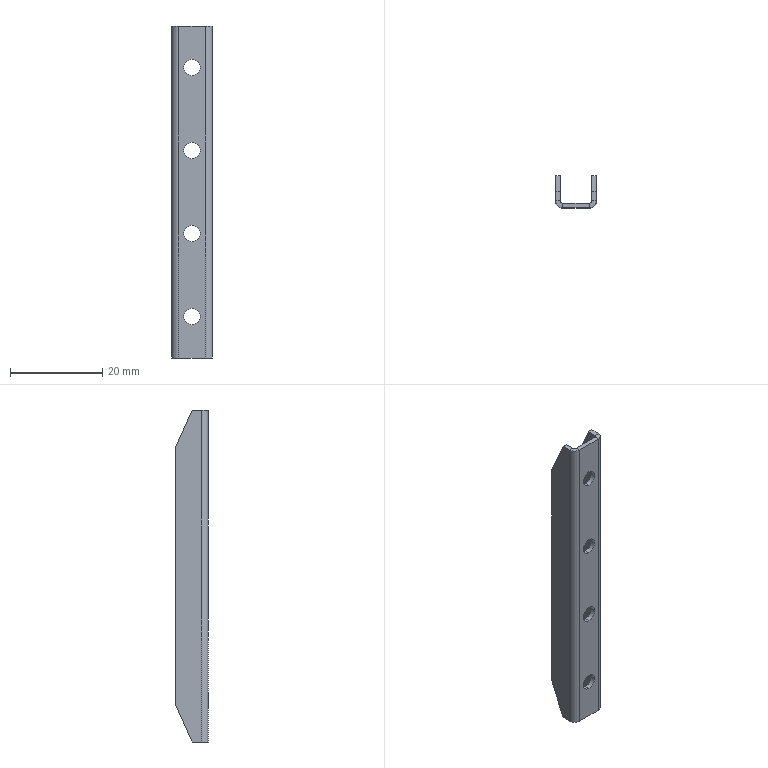Part | SolidWorks | features Chamfer 2, FlatPattern 1, HoleWzd 1, SMBaseFlange 1, SheetMetal 1 | 1 solid | 34 faces | box 8.8 x 7 x 72 mm | volume 1341 mm3 | plane 22 | cylinder 12 | commonest cylinder face diameters 3.5 x8 1 x2 3 x2
STEP:
#1=CARTESIAN_POINT('',(3.4,0.,25.25));
#2=VERTEX_POINT('',#1);
#3=CARTESIAN_POINT('',(3.4,0.,28.75));
#4=VERTEX_POINT('',#3);
#5=CARTESIAN_POINT('',(3.4,0.,27.));
#6=DIRECTION('',(0.,1.,0.));
#7=DIRECTION('',(0.,0.,1.));
#8=AXIS2_PLACEMENT_3D('',#5,#6,#7);
#9=CIRCLE('',#8,1.75);
#10=EDGE_CURVE('',#2,#4,#9,.T.);
#11=ORIENTED_EDGE('',*,*,#10,.T.);
#12=CARTESIAN_POINT('',(3.4,-1.,28.75));
#13=VERTEX_POINT('',#12);
#14=CARTESIAN_POINT('',(3.4,-1.,28.75));
#15=DIRECTION('',(0.,-1.,0.));
#16=VECTOR('',#15,1000.);
#17=LINE('',#14,#16);
#18=EDGE_CURVE('',#4,#13,#17,.T.);
#19=ORIENTED_EDGE('',*,*,#18,.T.);
#20=CARTESIAN_POINT('',(3.4,-1.,25.25));
#21=VERTEX_POINT('',#20);
#22=CARTESIAN_POINT('',(3.4,-1.,27.));
#23=DIRECTION('',(0.,-1.,0.));
#24=DIRECTION('',(0.,0.,-1.));
#25=AXIS2_PLACEMENT_3D('',#22,#23,#24);
#26=CIRCLE('',#25,1.75);
#27=EDGE_CURVE('',#13,#21,#26,.T.);
#28=ORIENTED_EDGE('',*,*,#27,.T.);
#29=CARTESIAN_POINT('',(3.4,-1.,25.25));
#30=DIRECTION('',(0.,-1.,0.));
#31=VECTOR('',#30,1000.);
#32=LINE('',#29,#31);
#33=EDGE_CURVE('',#2,#21,#32,.T.);
#34=ORIENTED_EDGE('',*,*,#33,.F.);
#35=EDGE_LOOP('',(#11,#19,#28,#34));
#36=FACE_OUTER_BOUND('',#35,.T.);
#37=CARTESIAN_POINT('',(3.4,-1.,27.));
#38=DIRECTION('',(0.,-1.,0.));
#39=DIRECTION('',(0.,0.,-1.));
#40=AXIS2_PLACEMENT_3D('',#37,#38,#39);
#41=CYLINDRICAL_SURFACE('',#40,1.75);
#42=ADVANCED_FACE('',(#36),#41,.F.);
#43=CARTESIAN_POINT('',(3.4,0.,7.25));
#44=VERTEX_POINT('',#43);
#45=CARTESIAN_POINT('',(3.4,0.,10.75));
#46=VERTEX_POINT('',#45);
#47=CARTESIAN_POINT('',(3.4,0.,9.));
#48=DIRECTION('',(0.,1.,0.));
#49=DIRECTION('',(0.,0.,1.));
#50=AXIS2_PLACEMENT_3D('',#47,#48,#49);
#51=CIRCLE('',#50,1.75);
#52=EDGE_CURVE('',#44,#46,#51,.T.);
#53=ORIENTED_EDGE('',*,*,#52,.T.);
#54=CARTESIAN_POINT('',(3.4,-1.,10.75));
#55=VERTEX_POINT('',#54);
#56=CARTESIAN_POINT('',(3.4,-1.,10.75));
#57=DIRECTION('',(0.,-1.,0.));
#58=VECTOR('',#57,1000.);
#59=LINE('',#56,#58);
#60=EDGE_CURVE('',#46,#55,#59,.T.);
#61=ORIENTED_EDGE('',*,*,#60,.T.);
#62=CARTESIAN_POINT('',(3.4,-1.,7.25));
#63=VERTEX_POINT('',#62);
#64=CARTESIAN_POINT('',(3.4,-1.,9.));
#65=DIRECTION('',(0.,-1.,0.));
#66=DIRECTION('',(0.,0.,-1.));
#67=AXIS2_PLACEMENT_3D('',#64,#65,#66);
#68=CIRCLE('',#67,1.75);
#69=EDGE_CURVE('',#55,#63,#68,.T.);
#70=ORIENTED_EDGE('',*,*,#69,.T.);
#71=CARTESIAN_POINT('',(3.4,-1.,7.25));
#72=DIRECTION('',(0.,-1.,0.));
#73=VECTOR('',#72,1000.);
#74=LINE('',#71,#73);
#75=EDGE_CURVE('',#44,#63,#74,.T.);
#76=ORIENTED_EDGE('',*,*,#75,.F.);
#77=EDGE_LOOP('',(#53,#61,#70,#76));
#78=FACE_OUTER_BOUND('',#77,.T.);
#79=CARTESIAN_POINT('',(3.4,-1.,9.));
#80=DIRECTION('',(0.,-1.,0.));
#81=DIRECTION('',(0.,0.,-1.));
#82=AXIS2_PLACEMENT_3D('',#79,#80,#81);
#83=CYLINDRICAL_SURFACE('',#82,1.75);
#84=ADVANCED_FACE('',(#78),#83,.F.);
#85=CARTESIAN_POINT('',(3.4,0.,-10.75));
#86=VERTEX_POINT('',#85);
#87=CARTESIAN_POINT('',(3.4,0.,-7.25));
#88=VERTEX_POINT('',#87);
#89=CARTESIAN_POINT('',(3.4,0.,-9.));
#90=DIRECTION('',(0.,1.,0.));
#91=DIRECTION('',(0.,0.,1.));
#92=AXIS2_PLACEMENT_3D('',#89,#90,#91);
#93=CIRCLE('',#92,1.75);
#94=EDGE_CURVE('',#86,#88,#93,.T.);
#95=ORIENTED_EDGE('',*,*,#94,.T.);
#96=CARTESIAN_POINT('',(3.4,-1.,-7.25));
#97=VERTEX_POINT('',#96);
#98=CARTESIAN_POINT('',(3.4,-1.,-7.25));
#99=DIRECTION('',(0.,-1.,0.));
#100=VECTOR('',#99,1000.);
#101=LINE('',#98,#100);
#102=EDGE_CURVE('',#88,#97,#101,.T.);
#103=ORIENTED_EDGE('',*,*,#102,.T.);
#104=CARTESIAN_POINT('',(3.4,-1.,-10.75));
#105=VERTEX_POINT('',#104);
#106=CARTESIAN_POINT('',(3.4,-1.,-9.));
#107=DIRECTION('',(0.,-1.,0.));
#108=DIRECTION('',(0.,0.,-1.));
#109=AXIS2_PLACEMENT_3D('',#106,#107,#108);
#110=CIRCLE('',#109,1.75);
#111=EDGE_CURVE('',#97,#105,#110,.T.);
#112=ORIENTED_EDGE('',*,*,#111,.T.);
#113=CARTESIAN_POINT('',(3.4,-1.,-10.75));
#114=DIRECTION('',(0.,-1.,0.));
#115=VECTOR('',#114,1000.);
#116=LINE('',#113,#115);
#117=EDGE_CURVE('',#86,#105,#116,.T.);
#118=ORIENTED_EDGE('',*,*,#117,.F.);
#119=EDGE_LOOP('',(#95,#103,#112,#118));
#120=FACE_OUTER_BOUND('',#119,.T.);
#121=CARTESIAN_POINT('',(3.4,-1.,-9.));
#122=DIRECTION('',(0.,-1.,0.));
#123=DIRECTION('',(0.,0.,-1.));
#124=AXIS2_PLACEMENT_3D('',#121,#122,#123);
#125=CYLINDRICAL_SURFACE('',#124,1.75);
#126=ADVANCED_FACE('',(#120),#125,.F.);
#127=CARTESIAN_POINT('',(3.4,0.,-28.75));
#128=VERTEX_POINT('',#127);
#129=CARTESIAN_POINT('',(3.4,0.,-25.25));
#130=VERTEX_POINT('',#129);
#131=CARTESIAN_POINT('',(3.4,0.,-27.));
#132=DIRECTION('',(0.,1.,0.));
#133=DIRECTION('',(0.,0.,1.));
#134=AXIS2_PLACEMENT_3D('',#131,#132,#133);
#135=CIRCLE('',#134,1.75);
#136=EDGE_CURVE('',#128,#130,#135,.T.);
#137=ORIENTED_EDGE('',*,*,#136,.T.);
#138=CARTESIAN_POINT('',(3.4,-1.,-25.25));
#139=VERTEX_POINT('',#138);
#140=CARTESIAN_POINT('',(3.4,-1.,-25.25));
#141=DIRECTION('',(0.,-1.,0.));
#142=VECTOR('',#141,1000.);
#143=LINE('',#140,#142);
#144=EDGE_CURVE('',#130,#139,#143,.T.);
#145=ORIENTED_EDGE('',*,*,#144,.T.);
#146=CARTESIAN_POINT('',(3.4,-1.,-28.75));
#147=VERTEX_POINT('',#146);
#148=CARTESIAN_POINT('',(3.4,-1.,-27.));
#149=DIRECTION('',(0.,-1.,0.));
#150=DIRECTION('',(0.,0.,-1.));
#151=AXIS2_PLACEMENT_3D('',#148,#149,#150);
#152=CIRCLE('',#151,1.75);
#153=EDGE_CURVE('',#139,#147,#152,.T.);
#154=ORIENTED_EDGE('',*,*,#153,.T.);
#155=CARTESIAN_POINT('',(3.4,-1.,-28.75));
#156=DIRECTION('',(0.,-1.,0.));
#157=VECTOR('',#156,1000.);
#158=LINE('',#155,#157);
#159=EDGE_CURVE('',#128,#147,#158,.T.);
#160=ORIENTED_EDGE('',*,*,#159,.F.);
#161=EDGE_LOOP('',(#137,#145,#154,#160));
#162=FACE_OUTER_BOUND('',#161,.T.);
#163=CARTESIAN_POINT('',(3.4,-1.,-27.));
#164=DIRECTION('',(0.,-1.,0.));
#165=DIRECTION('',(0.,0.,-1.));
#166=AXIS2_PLACEMENT_3D('',#163,#164,#165);
#167=CYLINDRICAL_SURFACE('',#166,1.75);
#168=ADVANCED_FACE('',(#162),#167,.F.);
#169=CARTESIAN_POINT('',(0.5,0.,36.));
#170=VERTEX_POINT('',#169);
#171=CARTESIAN_POINT('',(0.5,-1.,36.));
#172=VERTEX_POINT('',#171);
#173=CARTESIAN_POINT('',(0.5,0.,36.));
#174=DIRECTION('',(0.,-1.,0.));
#175=VECTOR('',#174,1000.);
#176=LINE('',#173,#175);
#177=EDGE_CURVE('',#170,#172,#176,.T.);
#178=ORIENTED_EDGE('',*,*,#177,.F.);
#179=CARTESIAN_POINT('',(0.,0.5,36.));
#180=VERTEX_POINT('',#179);
#181=CARTESIAN_POINT('',(0.5,0.5,36.));
#182=DIRECTION('',(0.,0.,1.));
#183=DIRECTION('',(-1.,0.,0.));
#184=AXIS2_PLACEMENT_3D('',#181,#182,#183);
#185=CIRCLE('',#184,0.5);
#186=EDGE_CURVE('',#180,#170,#185,.T.);
#187=ORIENTED_EDGE('',*,*,#186,.F.);
#188=CARTESIAN_POINT('',(-1.,0.5,36.));
#189=VERTEX_POINT('',#188);
#190=CARTESIAN_POINT('',(-1.,0.5,36.));
#191=DIRECTION('',(1.,0.,0.));
#192=VECTOR('',#191,1000.);
#193=LINE('',#190,#192);
#194=EDGE_CURVE('',#189,#180,#193,.T.);
#195=ORIENTED_EDGE('',*,*,#194,.F.);
#196=CARTESIAN_POINT('',(0.5,0.5,36.));
#197=DIRECTION('',(0.,0.,1.));
#198=DIRECTION('',(1.,0.,0.));
#199=AXIS2_PLACEMENT_3D('',#196,#197,#198);
#200=CIRCLE('',#199,1.5);
#201=EDGE_CURVE('',#189,#172,#200,.T.);
#202=ORIENTED_EDGE('',*,*,#201,.T.);
#203=EDGE_LOOP('',(#178,#187,#195,#202));
#204=FACE_OUTER_BOUND('',#203,.T.);
#205=CARTESIAN_POINT('',(0.5,0.,36.));
#206=DIRECTION('',(0.,0.,1.));
#207=DIRECTION('',(1.,0.,0.));
#208=AXIS2_PLACEMENT_3D('',#205,#206,#207);
#209=PLANE('',#208);
#210=ADVANCED_FACE('',(#204),#209,.T.);
#211=CARTESIAN_POINT('',(6.3,0.,36.));
#212=VERTEX_POINT('',#211);
#213=CARTESIAN_POINT('',(0.,0.,36.));
#214=DIRECTION('',(1.,0.,0.));
#215=VECTOR('',#214,1000.);
#216=LINE('',#213,#215);
#217=EDGE_CURVE('',#170,#212,#216,.T.);
#218=ORIENTED_EDGE('',*,*,#217,.F.);
#219=ORIENTED_EDGE('',*,*,#177,.T.);
#220=CARTESIAN_POINT('',(6.3,-1.,36.));
#221=VERTEX_POINT('',#220);
#222=CARTESIAN_POINT('',(0.,-1.,36.));
#223=DIRECTION('',(1.,0.,0.));
#224=VECTOR('',#223,1000.);
#225=LINE('',#222,#224);
#226=EDGE_CURVE('',#172,#221,#225,.T.);
#227=ORIENTED_EDGE('',*,*,#226,.T.);
#228=CARTESIAN_POINT('',(6.3,-1.,36.));
#229=DIRECTION('',(0.,1.,0.));
#230=VECTOR('',#229,1000.);
#231=LINE('',#228,#230);
#232=EDGE_CURVE('',#221,#212,#231,.T.);
#233=ORIENTED_EDGE('',*,*,#232,.T.);
#234=EDGE_LOOP('',(#218,#219,#227,#233));
#235=FACE_OUTER_BOUND('',#234,.T.);
#236=CARTESIAN_POINT('',(-1.,0.5,36.));
#237=DIRECTION('',(0.,0.,1.));
#238=DIRECTION('',(1.,0.,0.));
#239=AXIS2_PLACEMENT_3D('',#236,#237,#238);
#240=PLANE('',#239);
#241=ADVANCED_FACE('',(#235),#240,.T.);
#242=CARTESIAN_POINT('',(0.,0.5,-36.));
#243=VERTEX_POINT('',#242);
#244=CARTESIAN_POINT('',(-1.,0.5,-36.));
#245=VERTEX_POINT('',#244);
#246=CARTESIAN_POINT('',(0.,0.5,-36.));
#247=DIRECTION('',(-1.,0.,0.));
#248=VECTOR('',#247,1000.);
#249=LINE('',#246,#248);
#250=EDGE_CURVE('',#243,#245,#249,.T.);
#251=ORIENTED_EDGE('',*,*,#250,.F.);
#252=CARTESIAN_POINT('',(0.5,0.,-36.));
#253=VERTEX_POINT('',#252);
#254=CARTESIAN_POINT('',(0.5,0.5,-36.));
#255=DIRECTION('',(0.,0.,1.));
#256=DIRECTION('',(-1.,0.,0.));
#257=AXIS2_PLACEMENT_3D('',#254,#255,#256);
#258=CIRCLE('',#257,0.5);
#259=EDGE_CURVE('',#243,#253,#258,.T.);
#260=ORIENTED_EDGE('',*,*,#259,.T.);
#261=CARTESIAN_POINT('',(0.5,-1.,-36.));
#262=VERTEX_POINT('',#261);
#263=CARTESIAN_POINT('',(0.5,-1.,-36.));
#264=DIRECTION('',(0.,1.,0.));
#265=VECTOR('',#264,1000.);
#266=LINE('',#263,#265);
#267=EDGE_CURVE('',#262,#253,#266,.T.);
#268=ORIENTED_EDGE('',*,*,#267,.F.);
#269=CARTESIAN_POINT('',(0.5,0.5,-36.));
#270=DIRECTION('',(0.,0.,1.));
#271=DIRECTION('',(1.,0.,0.));
#272=AXIS2_PLACEMENT_3D('',#269,#270,#271);
#273=CIRCLE('',#272,1.5);
#274=EDGE_CURVE('',#245,#262,#273,.T.);
#275=ORIENTED_EDGE('',*,*,#274,.F.);
#276=EDGE_LOOP('',(#251,#260,#268,#275));
#277=FACE_OUTER_BOUND('',#276,.T.);
#278=CARTESIAN_POINT('',(0.,0.5,-36.));
#279=DIRECTION('',(0.,0.,-1.));
#280=DIRECTION('',(-1.,0.,0.));
#281=AXIS2_PLACEMENT_3D('',#278,#279,#280);
#282=PLANE('',#281);
#283=ADVANCED_FACE('',(#277),#282,.T.);
#284=CARTESIAN_POINT('',(-1.,2.5,-36.));
#285=VERTEX_POINT('',#284);
#286=CARTESIAN_POINT('',(-1.,0.,-36.));
#287=DIRECTION('',(0.,-1.,0.));
#288=VECTOR('',#287,1000.);
#289=LINE('',#286,#288);
#290=EDGE_CURVE('',#285,#245,#289,.T.);
#291=ORIENTED_EDGE('',*,*,#290,.F.);
#292=CARTESIAN_POINT('',(0.,2.5,-36.));
#293=VERTEX_POINT('',#292);
#294=CARTESIAN_POINT('',(0.5,2.5,-36.));
#295=DIRECTION('',(1.,0.,0.));
#296=VECTOR('',#295,1000.);
#297=LINE('',#294,#296);
#298=EDGE_CURVE('',#285,#293,#297,.T.);
#299=ORIENTED_EDGE('',*,*,#298,.T.);
#300=CARTESIAN_POINT('',(0.,0.,-36.));
#301=DIRECTION('',(0.,-1.,0.));
#302=VECTOR('',#301,1000.);
#303=LINE('',#300,#302);
#304=EDGE_CURVE('',#293,#243,#303,.T.);
#305=ORIENTED_EDGE('',*,*,#304,.T.);
#306=ORIENTED_EDGE('',*,*,#250,.T.);
#307=EDGE_LOOP('',(#291,#299,#305,#306));
#308=FACE_OUTER_BOUND('',#307,.T.);
#309=CARTESIAN_POINT('',(0.5,-1.,-36.));
#310=DIRECTION('',(0.,0.,-1.));
#311=DIRECTION('',(-1.,0.,0.));
#312=AXIS2_PLACEMENT_3D('',#309,#310,#311);
#313=PLANE('',#312);
#314=ADVANCED_FACE('',(#308),#313,.T.);
#315=CARTESIAN_POINT('',(6.8,0.5,36.));
#316=VERTEX_POINT('',#315);
#317=CARTESIAN_POINT('',(7.8,0.5,36.));
#318=VERTEX_POINT('',#317);
#319=CARTESIAN_POINT('',(6.8,0.5,36.));
#320=DIRECTION('',(1.,0.,0.));
#321=VECTOR('',#320,1000.);
#322=LINE('',#319,#321);
#323=EDGE_CURVE('',#316,#318,#322,.T.);
#324=ORIENTED_EDGE('',*,*,#323,.F.);
#325=CARTESIAN_POINT('',(6.3,0.5,36.));
#326=DIRECTION('',(0.,0.,1.));
#327=DIRECTION('',(-1.,0.,0.));
#328=AXIS2_PLACEMENT_3D('',#325,#326,#327);
#329=CIRCLE('',#328,0.5);
#330=EDGE_CURVE('',#212,#316,#329,.T.);
#331=ORIENTED_EDGE('',*,*,#330,.F.);
#332=ORIENTED_EDGE('',*,*,#232,.F.);
#333=CARTESIAN_POINT('',(6.3,0.5,36.));
#334=DIRECTION('',(0.,0.,1.));
#335=DIRECTION('',(1.,0.,0.));
#336=AXIS2_PLACEMENT_3D('',#333,#334,#335);
#337=CIRCLE('',#336,1.5);
#338=EDGE_CURVE('',#221,#318,#337,.T.);
#339=ORIENTED_EDGE('',*,*,#338,.T.);
#340=EDGE_LOOP('',(#324,#331,#332,#339));
#341=FACE_OUTER_BOUND('',#340,.T.);
#342=CARTESIAN_POINT('',(6.8,0.5,36.));
#343=DIRECTION('',(0.,0.,1.));
#344=DIRECTION('',(1.,0.,0.));
#345=AXIS2_PLACEMENT_3D('',#342,#343,#344);
#346=PLANE('',#345);
#347=ADVANCED_FACE('',(#341),#346,.T.);
#348=CARTESIAN_POINT('',(7.8,2.5,36.));
#349=VERTEX_POINT('',#348);
#350=CARTESIAN_POINT('',(7.8,0.,36.));
#351=DIRECTION('',(0.,1.,0.));
#352=VECTOR('',#351,1000.);
#353=LINE('',#350,#352);
#354=EDGE_CURVE('',#318,#349,#353,.T.);
#355=ORIENTED_EDGE('',*,*,#354,.T.);
#356=CARTESIAN_POINT('',(6.8,2.5,36.));
#357=VERTEX_POINT('',#356);
#358=CARTESIAN_POINT('',(6.3,2.5,36.));
#359=DIRECTION('',(-1.,0.,0.));
#360=VECTOR('',#359,1000.);
#361=LINE('',#358,#360);
#362=EDGE_CURVE('',#349,#357,#361,.T.);
#363=ORIENTED_EDGE('',*,*,#362,.T.);
#364=CARTESIAN_POINT('',(6.8,0.,36.));
#365=DIRECTION('',(0.,1.,0.));
#366=VECTOR('',#365,1000.);
#367=LINE('',#364,#366);
#368=EDGE_CURVE('',#316,#357,#367,.T.);
#369=ORIENTED_EDGE('',*,*,#368,.F.);
#370=ORIENTED_EDGE('',*,*,#323,.T.);
#371=EDGE_LOOP('',(#355,#363,#369,#370));
#372=FACE_OUTER_BOUND('',#371,.T.);
#373=CARTESIAN_POINT('',(6.3,-1.,36.));
#374=DIRECTION('',(0.,0.,1.));
#375=DIRECTION('',(1.,0.,0.));
#376=AXIS2_PLACEMENT_3D('',#373,#374,#375);
#377=PLANE('',#376);
#378=ADVANCED_FACE('',(#372),#377,.T.);
#379=CARTESIAN_POINT('',(6.3,0.,-36.));
#380=VERTEX_POINT('',#379);
#381=CARTESIAN_POINT('',(6.3,-1.,-36.));
#382=VERTEX_POINT('',#381);
#383=CARTESIAN_POINT('',(6.3,0.,-36.));
#384=DIRECTION('',(0.,-1.,0.));
#385=VECTOR('',#384,1000.);
#386=LINE('',#383,#385);
#387=EDGE_CURVE('',#380,#382,#386,.T.);
#388=ORIENTED_EDGE('',*,*,#387,.F.);
#389=CARTESIAN_POINT('',(6.8,0.5,-36.));
#390=VERTEX_POINT('',#389);
#391=CARTESIAN_POINT('',(6.3,0.5,-36.));
#392=DIRECTION('',(0.,0.,1.));
#393=DIRECTION('',(-1.,0.,0.));
#394=AXIS2_PLACEMENT_3D('',#391,#392,#393);
#395=CIRCLE('',#394,0.5);
#396=EDGE_CURVE('',#380,#390,#395,.T.);
#397=ORIENTED_EDGE('',*,*,#396,.T.);
#398=CARTESIAN_POINT('',(7.8,0.5,-36.));
#399=VERTEX_POINT('',#398);
#400=CARTESIAN_POINT('',(7.8,0.5,-36.));
#401=DIRECTION('',(-1.,0.,0.));
#402=VECTOR('',#401,1000.);
#403=LINE('',#400,#402);
#404=EDGE_CURVE('',#399,#390,#403,.T.);
#405=ORIENTED_EDGE('',*,*,#404,.F.);
#406=CARTESIAN_POINT('',(6.3,0.5,-36.));
#407=DIRECTION('',(0.,0.,1.));
#408=DIRECTION('',(1.,0.,0.));
#409=AXIS2_PLACEMENT_3D('',#406,#407,#408);
#410=CIRCLE('',#409,1.5);
#411=EDGE_CURVE('',#382,#399,#410,.T.);
#412=ORIENTED_EDGE('',*,*,#411,.F.);
#413=EDGE_LOOP('',(#388,#397,#405,#412));
#414=FACE_OUTER_BOUND('',#413,.T.);
#415=CARTESIAN_POINT('',(6.3,0.,-36.));
#416=DIRECTION('',(0.,0.,-1.));
#417=DIRECTION('',(-1.,0.,0.));
#418=AXIS2_PLACEMENT_3D('',#415,#416,#417);
#419=PLANE('',#418);
#420=ADVANCED_FACE('',(#414),#419,.T.);
#421=CARTESIAN_POINT('',(0.,0.,-36.));
#422=DIRECTION('',(1.,0.,0.));
#423=VECTOR('',#422,1000.);
#424=LINE('',#421,#423);
#425=EDGE_CURVE('',#253,#380,#424,.T.);
#426=ORIENTED_EDGE('',*,*,#425,.T.);
#427=ORIENTED_EDGE('',*,*,#387,.T.);
#428=CARTESIAN_POINT('',(0.,-1.,-36.));
#429=DIRECTION('',(1.,0.,0.));
#430=VECTOR('',#429,1000.);
#431=LINE('',#428,#430);
#432=EDGE_CURVE('',#262,#382,#431,.T.);
#433=ORIENTED_EDGE('',*,*,#432,.F.);
#434=ORIENTED_EDGE('',*,*,#267,.T.);
#435=EDGE_LOOP('',(#426,#427,#433,#434));
#436=FACE_OUTER_BOUND('',#435,.T.);
#437=CARTESIAN_POINT('',(7.8,0.5,-36.));
#438=DIRECTION('',(0.,0.,-1.));
#439=DIRECTION('',(-1.,0.,0.));
#440=AXIS2_PLACEMENT_3D('',#437,#438,#439);
#441=PLANE('',#440);
#442=ADVANCED_FACE('',(#436),#441,.T.);
#443=CARTESIAN_POINT('',(7.8,2.5,-36.));
#444=VERTEX_POINT('',#443);
#445=CARTESIAN_POINT('',(7.8,0.,-36.));
#446=DIRECTION('',(0.,1.,0.));
#447=VECTOR('',#446,1000.);
#448=LINE('',#445,#447);
#449=EDGE_CURVE('',#399,#444,#448,.T.);
#450=ORIENTED_EDGE('',*,*,#449,.T.);
#451=CARTESIAN_POINT('',(7.8,6.,-28.));
#452=VERTEX_POINT('',#451);
#453=CARTESIAN_POINT('',(7.8,2.5,-36.));
#454=DIRECTION('',(0.,0.4008,0.9162));
#455=VECTOR('',#454,1000.);
#456=LINE('',#453,#455);
#457=EDGE_CURVE('',#444,#452,#456,.T.);
#458=ORIENTED_EDGE('',*,*,#457,.T.);
#459=CARTESIAN_POINT('',(7.8,6.,28.));
#460=VERTEX_POINT('',#459);
#461=CARTESIAN_POINT('',(7.8,6.,36.));
#462=DIRECTION('',(0.,0.,-1.));
#463=VECTOR('',#462,1000.);
#464=LINE('',#461,#463);
#465=EDGE_CURVE('',#460,#452,#464,.T.);
#466=ORIENTED_EDGE('',*,*,#465,.F.);
#467=CARTESIAN_POINT('',(7.8,6.,28.));
#468=DIRECTION('',(0.,-0.4008,0.9162));
#469=VECTOR('',#468,1000.);
#470=LINE('',#467,#469);
#471=EDGE_CURVE('',#460,#349,#470,.T.);
#472=ORIENTED_EDGE('',*,*,#471,.T.);
#473=ORIENTED_EDGE('',*,*,#354,.F.);
#474=CARTESIAN_POINT('',(7.8,0.5,36.));
#475=DIRECTION('',(0.,0.,-1.));
#476=VECTOR('',#475,1000.);
#477=LINE('',#474,#476);
#478=EDGE_CURVE('',#318,#399,#477,.T.);
#479=ORIENTED_EDGE('',*,*,#478,.T.);
#480=EDGE_LOOP('',(#450,#458,#466,#472,#473,#479));
#481=FACE_OUTER_BOUND('',#480,.T.);
#482=CARTESIAN_POINT('',(7.8,0.,36.));
#483=DIRECTION('',(-1.,0.,0.));
#484=DIRECTION('',(0.,0.,1.));
#485=AXIS2_PLACEMENT_3D('',#482,#483,#484);
#486=PLANE('',#485);
#487=ADVANCED_FACE('',(#481),#486,.F.);
#488=ORIENTED_EDGE('',*,*,#465,.T.);
#489=CARTESIAN_POINT('',(6.8,6.,-28.));
#490=VERTEX_POINT('',#489);
#491=CARTESIAN_POINT('',(6.8,6.,-28.));
#492=DIRECTION('',(-1.,0.,0.));
#493=VECTOR('',#492,1000.);
#494=LINE('',#491,#493);
#495=EDGE_CURVE('',#452,#490,#494,.T.);
#496=ORIENTED_EDGE('',*,*,#495,.T.);
#497=CARTESIAN_POINT('',(6.8,6.,28.));
#498=VERTEX_POINT('',#497);
#499=CARTESIAN_POINT('',(6.8,6.,36.));
#500=DIRECTION('',(0.,0.,-1.));
#501=VECTOR('',#500,1000.);
#502=LINE('',#499,#501);
#503=EDGE_CURVE('',#498,#490,#502,.T.);
#504=ORIENTED_EDGE('',*,*,#503,.F.);
#505=CARTESIAN_POINT('',(6.8,6.,28.));
#506=DIRECTION('',(1.,0.,0.));
#507=VECTOR('',#506,1000.);
#508=LINE('',#505,#507);
#509=EDGE_CURVE('',#498,#460,#508,.T.);
#510=ORIENTED_EDGE('',*,*,#509,.T.);
#511=EDGE_LOOP('',(#488,#496,#504,#510));
#512=FACE_OUTER_BOUND('',#511,.T.);
#513=CARTESIAN_POINT('',(6.8,6.,36.));
#514=DIRECTION('',(0.,1.,0.));
#515=DIRECTION('',(0.,0.,1.));
#516=AXIS2_PLACEMENT_3D('',#513,#514,#515);
#517=PLANE('',#516);
#518=ADVANCED_FACE('',(#512),#517,.T.);
#519=ORIENTED_EDGE('',*,*,#503,.T.);
#520=CARTESIAN_POINT('',(6.8,2.5,-36.));
#521=VERTEX_POINT('',#520);
#522=CARTESIAN_POINT('',(6.8,28.538,23.515));
#523=DIRECTION('',(0.,-0.4008,-0.9162));
#524=VECTOR('',#523,1000.);
#525=LINE('',#522,#524);
#526=EDGE_CURVE('',#490,#521,#525,.T.);
#527=ORIENTED_EDGE('',*,*,#526,.T.);
#528=CARTESIAN_POINT('',(6.8,0.,-36.));
#529=DIRECTION('',(0.,1.,0.));
#530=VECTOR('',#529,1000.);
#531=LINE('',#528,#530);
#532=EDGE_CURVE('',#390,#521,#531,.T.);
#533=ORIENTED_EDGE('',*,*,#532,.F.);
#534=CARTESIAN_POINT('',(6.8,0.5,36.));
#535=DIRECTION('',(0.,0.,-1.));
#536=VECTOR('',#535,1000.);
#537=LINE('',#534,#536);
#538=EDGE_CURVE('',#316,#390,#537,.T.);
#539=ORIENTED_EDGE('',*,*,#538,.F.);
#540=ORIENTED_EDGE('',*,*,#368,.T.);
#541=CARTESIAN_POINT('',(6.8,2.098,36.918));
#542=DIRECTION('',(0.,0.4008,-0.9162));
#543=VECTOR('',#542,1000.);
#544=LINE('',#541,#543);
#545=EDGE_CURVE('',#357,#498,#544,.T.);
#546=ORIENTED_EDGE('',*,*,#545,.T.);
#547=EDGE_LOOP('',(#519,#527,#533,#539,#540,#546));
#548=FACE_OUTER_BOUND('',#547,.T.);
#549=CARTESIAN_POINT('',(6.8,0.,36.));
#550=DIRECTION('',(-1.,0.,0.));
#551=DIRECTION('',(0.,0.,1.));
#552=AXIS2_PLACEMENT_3D('',#549,#550,#551);
#553=PLANE('',#552);
#554=ADVANCED_FACE('',(#548),#553,.T.);
#555=ORIENTED_EDGE('',*,*,#396,.F.);
#556=CARTESIAN_POINT('',(6.3,0.,36.));
#557=DIRECTION('',(0.,0.,-1.));
#558=VECTOR('',#557,1000.);
#559=LINE('',#556,#558);
#560=EDGE_CURVE('',#212,#380,#559,.T.);
#561=ORIENTED_EDGE('',*,*,#560,.F.);
#562=ORIENTED_EDGE('',*,*,#330,.T.);
#563=ORIENTED_EDGE('',*,*,#538,.T.);
#564=EDGE_LOOP('',(#555,#561,#562,#563));
#565=FACE_OUTER_BOUND('',#564,.T.);
#566=CARTESIAN_POINT('',(6.3,0.5,36.));
#567=DIRECTION('',(0.,0.,-1.));
#568=DIRECTION('',(-1.,0.,0.));
#569=AXIS2_PLACEMENT_3D('',#566,#567,#568);
#570=CYLINDRICAL_SURFACE('',#569,0.5);
#571=ADVANCED_FACE('',(#565),#570,.F.);
#572=ORIENTED_EDGE('',*,*,#10,.F.);
#573=CARTESIAN_POINT('',(3.4,0.,27.));
#574=DIRECTION('',(0.,1.,0.));
#575=DIRECTION('',(0.,0.,1.));
#576=AXIS2_PLACEMENT_3D('',#573,#574,#575);
#577=CIRCLE('',#576,1.75);
#578=EDGE_CURVE('',#4,#2,#577,.T.);
#579=ORIENTED_EDGE('',*,*,#578,.F.);
#580=EDGE_LOOP('',(#572,#579));
#581=FACE_BOUND('',#580,.T.);
#582=ORIENTED_EDGE('',*,*,#52,.F.);
#583=CARTESIAN_POINT('',(3.4,0.,9.));
#584=DIRECTION('',(0.,1.,0.));
#585=DIRECTION('',(0.,0.,1.));
#586=AXIS2_PLACEMENT_3D('',#583,#584,#585);
#587=CIRCLE('',#586,1.75);
#588=EDGE_CURVE('',#46,#44,#587,.T.);
#589=ORIENTED_EDGE('',*,*,#588,.F.);
#590=EDGE_LOOP('',(#582,#589));
#591=FACE_BOUND('',#590,.T.);
#592=ORIENTED_EDGE('',*,*,#94,.F.);
#593=CARTESIAN_POINT('',(3.4,0.,-9.));
#594=DIRECTION('',(0.,1.,0.));
#595=DIRECTION('',(0.,0.,1.));
#596=AXIS2_PLACEMENT_3D('',#593,#594,#595);
#597=CIRCLE('',#596,1.75);
#598=EDGE_CURVE('',#88,#86,#597,.T.);
#599=ORIENTED_EDGE('',*,*,#598,.F.);
#600=EDGE_LOOP('',(#592,#599));
#601=FACE_BOUND('',#600,.T.);
#602=ORIENTED_EDGE('',*,*,#136,.F.);
#603=CARTESIAN_POINT('',(3.4,0.,-27.));
#604=DIRECTION('',(0.,1.,0.));
#605=DIRECTION('',(0.,0.,1.));
#606=AXIS2_PLACEMENT_3D('',#603,#604,#605);
#607=CIRCLE('',#606,1.75);
#608=EDGE_CURVE('',#130,#128,#607,.T.);
#609=ORIENTED_EDGE('',*,*,#608,.F.);
#610=EDGE_LOOP('',(#602,#609));
#611=FACE_BOUND('',#610,.T.);
#612=ORIENTED_EDGE('',*,*,#425,.F.);
#613=CARTESIAN_POINT('',(0.5,0.,36.));
#614=DIRECTION('',(0.,0.,-1.));
#615=VECTOR('',#614,1000.);
#616=LINE('',#613,#615);
#617=EDGE_CURVE('',#170,#253,#616,.T.);
#618=ORIENTED_EDGE('',*,*,#617,.F.);
#619=ORIENTED_EDGE('',*,*,#217,.T.);
#620=ORIENTED_EDGE('',*,*,#560,.T.);
#621=EDGE_LOOP('',(#612,#618,#619,#620));
#622=FACE_OUTER_BOUND('',#621,.T.);
#623=CARTESIAN_POINT('',(0.,0.,36.));
#624=DIRECTION('',(0.,1.,0.));
#625=DIRECTION('',(0.,0.,1.));
#626=AXIS2_PLACEMENT_3D('',#623,#624,#625);
#627=PLANE('',#626);
#628=ADVANCED_FACE('',(#581,#591,#601,#611,#622),#627,.T.);
#629=ORIENTED_EDGE('',*,*,#259,.F.);
#630=CARTESIAN_POINT('',(0.,0.5,36.));
#631=DIRECTION('',(0.,0.,-1.));
#632=VECTOR('',#631,1000.);
#633=LINE('',#630,#632);
#634=EDGE_CURVE('',#180,#243,#633,.T.);
#635=ORIENTED_EDGE('',*,*,#634,.F.);
#636=ORIENTED_EDGE('',*,*,#186,.T.);
#637=ORIENTED_EDGE('',*,*,#617,.T.);
#638=EDGE_LOOP('',(#629,#635,#636,#637));
#639=FACE_OUTER_BOUND('',#638,.T.);
#640=CARTESIAN_POINT('',(0.5,0.5,36.));
#641=DIRECTION('',(0.,0.,-1.));
#642=DIRECTION('',(-1.,0.,0.));
#643=AXIS2_PLACEMENT_3D('',#640,#641,#642);
#644=CYLINDRICAL_SURFACE('',#643,0.5);
#645=ADVANCED_FACE('',(#639),#644,.F.);
#646=ORIENTED_EDGE('',*,*,#304,.F.);
#647=CARTESIAN_POINT('',(0.,6.,-28.));
#648=VERTEX_POINT('',#647);
#649=CARTESIAN_POINT('',(0.,28.538,23.515));
#650=DIRECTION('',(0.,0.4008,0.9162));
#651=VECTOR('',#650,1000.);
#652=LINE('',#649,#651);
#653=EDGE_CURVE('',#293,#648,#652,.T.);
#654=ORIENTED_EDGE('',*,*,#653,.T.);
#655=CARTESIAN_POINT('',(0.,6.,28.));
#656=VERTEX_POINT('',#655);
#657=CARTESIAN_POINT('',(0.,6.,36.));
#658=DIRECTION('',(0.,0.,-1.));
#659=VECTOR('',#658,1000.);
#660=LINE('',#657,#659);
#661=EDGE_CURVE('',#656,#648,#660,.T.);
#662=ORIENTED_EDGE('',*,*,#661,.F.);
#663=CARTESIAN_POINT('',(0.,2.5,36.));
#664=VERTEX_POINT('',#663);
#665=CARTESIAN_POINT('',(0.,2.098,36.918));
#666=DIRECTION('',(0.,-0.4008,0.9162));
#667=VECTOR('',#666,1000.);
#668=LINE('',#665,#667);
#669=EDGE_CURVE('',#656,#664,#668,.T.);
#670=ORIENTED_EDGE('',*,*,#669,.T.);
#671=CARTESIAN_POINT('',(0.,0.,36.));
#672=DIRECTION('',(0.,-1.,0.));
#673=VECTOR('',#672,1000.);
#674=LINE('',#671,#673);
#675=EDGE_CURVE('',#664,#180,#674,.T.);
#676=ORIENTED_EDGE('',*,*,#675,.T.);
#677=ORIENTED_EDGE('',*,*,#634,.T.);
#678=EDGE_LOOP('',(#646,#654,#662,#670,#676,#677));
#679=FACE_OUTER_BOUND('',#678,.T.);
#680=CARTESIAN_POINT('',(0.,0.,36.));
#681=DIRECTION('',(1.,0.,0.));
#682=DIRECTION('',(0.,0.,-1.));
#683=AXIS2_PLACEMENT_3D('',#680,#681,#682);
#684=PLANE('',#683);
#685=ADVANCED_FACE('',(#679),#684,.T.);
#686=ORIENTED_EDGE('',*,*,#661,.T.);
#687=CARTESIAN_POINT('',(-1.,6.,-28.));
#688=VERTEX_POINT('',#687);
#689=CARTESIAN_POINT('',(-1.,6.,-28.));
#690=DIRECTION('',(-1.,0.,0.));
#691=VECTOR('',#690,1000.);
#692=LINE('',#689,#691);
#693=EDGE_CURVE('',#648,#688,#692,.T.);
#694=ORIENTED_EDGE('',*,*,#693,.T.);
#695=CARTESIAN_POINT('',(-1.,6.,28.));
#696=VERTEX_POINT('',#695);
#697=CARTESIAN_POINT('',(-1.,6.,36.));
#698=DIRECTION('',(0.,0.,-1.));
#699=VECTOR('',#698,1000.);
#700=LINE('',#697,#699);
#701=EDGE_CURVE('',#696,#688,#700,.T.);
#702=ORIENTED_EDGE('',*,*,#701,.F.);
#703=CARTESIAN_POINT('',(0.,6.,28.));
#704=DIRECTION('',(1.,0.,0.));
#705=VECTOR('',#704,1000.);
#706=LINE('',#703,#705);
#707=EDGE_CURVE('',#696,#656,#706,.T.);
#708=ORIENTED_EDGE('',*,*,#707,.T.);
#709=EDGE_LOOP('',(#686,#694,#702,#708));
#710=FACE_OUTER_BOUND('',#709,.T.);
#711=CARTESIAN_POINT('',(-1.,6.,36.));
#712=DIRECTION('',(0.,1.,0.));
#713=DIRECTION('',(0.,0.,1.));
#714=AXIS2_PLACEMENT_3D('',#711,#712,#713);
#715=PLANE('',#714);
#716=ADVANCED_FACE('',(#710),#715,.T.);
#717=ORIENTED_EDGE('',*,*,#701,.T.);
#718=CARTESIAN_POINT('',(-1.,2.5,-36.));
#719=DIRECTION('',(0.,-0.4008,-0.9162));
#720=VECTOR('',#719,1000.);
#721=LINE('',#718,#720);
#722=EDGE_CURVE('',#688,#285,#721,.T.);
#723=ORIENTED_EDGE('',*,*,#722,.T.);
#724=ORIENTED_EDGE('',*,*,#290,.T.);
#725=CARTESIAN_POINT('',(-1.,0.5,36.));
#726=DIRECTION('',(0.,0.,-1.));
#727=VECTOR('',#726,1000.);
#728=LINE('',#725,#727);
#729=EDGE_CURVE('',#189,#245,#728,.T.);
#730=ORIENTED_EDGE('',*,*,#729,.F.);
#731=CARTESIAN_POINT('',(-1.,2.5,36.));
#732=VERTEX_POINT('',#731);
#733=CARTESIAN_POINT('',(-1.,0.,36.));
#734=DIRECTION('',(0.,-1.,0.));
#735=VECTOR('',#734,1000.);
#736=LINE('',#733,#735);
#737=EDGE_CURVE('',#732,#189,#736,.T.);
#738=ORIENTED_EDGE('',*,*,#737,.F.);
#739=CARTESIAN_POINT('',(-1.,6.,28.));
#740=DIRECTION('',(0.,0.4008,-0.9162));
#741=VECTOR('',#740,1000.);
#742=LINE('',#739,#741);
#743=EDGE_CURVE('',#732,#696,#742,.T.);
#744=ORIENTED_EDGE('',*,*,#743,.T.);
#745=EDGE_LOOP('',(#717,#723,#724,#730,#738,#744));
#746=FACE_OUTER_BOUND('',#745,.T.);
#747=CARTESIAN_POINT('',(-1.,0.,36.));
#748=DIRECTION('',(1.,0.,0.));
#749=DIRECTION('',(0.,0.,-1.));
#750=AXIS2_PLACEMENT_3D('',#747,#748,#749);
#751=PLANE('',#750);
#752=ADVANCED_FACE('',(#746),#751,.F.);
#753=ORIENTED_EDGE('',*,*,#274,.T.);
#754=CARTESIAN_POINT('',(0.5,-1.,36.));
#755=DIRECTION('',(0.,0.,-1.));
#756=VECTOR('',#755,1000.);
#757=LINE('',#754,#756);
#758=EDGE_CURVE('',#172,#262,#757,.T.);
#759=ORIENTED_EDGE('',*,*,#758,.F.);
#760=ORIENTED_EDGE('',*,*,#201,.F.);
#761=ORIENTED_EDGE('',*,*,#729,.T.);
#762=EDGE_LOOP('',(#753,#759,#760,#761));
#763=FACE_OUTER_BOUND('',#762,.T.);
#764=CARTESIAN_POINT('',(0.5,0.5,36.));
#765=DIRECTION('',(0.,0.,-1.));
#766=DIRECTION('',(-1.,0.,0.));
#767=AXIS2_PLACEMENT_3D('',#764,#765,#766);
#768=CYLINDRICAL_SURFACE('',#767,1.5);
#769=ADVANCED_FACE('',(#763),#768,.T.);
#770=CARTESIAN_POINT('',(3.4,-1.,27.));
#771=DIRECTION('',(0.,-1.,0.));
#772=DIRECTION('',(0.,0.,-1.));
#773=AXIS2_PLACEMENT_3D('',#770,#771,#772);
#774=CIRCLE('',#773,1.75);
#775=EDGE_CURVE('',#21,#13,#774,.T.);
#776=ORIENTED_EDGE('',*,*,#775,.F.);
#777=ORIENTED_EDGE('',*,*,#27,.F.);
#778=EDGE_LOOP('',(#776,#777));
#779=FACE_BOUND('',#778,.T.);
#780=CARTESIAN_POINT('',(3.4,-1.,9.));
#781=DIRECTION('',(0.,-1.,0.));
#782=DIRECTION('',(0.,0.,-1.));
#783=AXIS2_PLACEMENT_3D('',#780,#781,#782);
#784=CIRCLE('',#783,1.75);
#785=EDGE_CURVE('',#63,#55,#784,.T.);
#786=ORIENTED_EDGE('',*,*,#785,.F.);
#787=ORIENTED_EDGE('',*,*,#69,.F.);
#788=EDGE_LOOP('',(#786,#787));
#789=FACE_BOUND('',#788,.T.);
#790=CARTESIAN_POINT('',(3.4,-1.,-9.));
#791=DIRECTION('',(0.,-1.,0.));
#792=DIRECTION('',(0.,0.,-1.));
#793=AXIS2_PLACEMENT_3D('',#790,#791,#792);
#794=CIRCLE('',#793,1.75);
#795=EDGE_CURVE('',#105,#97,#794,.T.);
#796=ORIENTED_EDGE('',*,*,#795,.F.);
#797=ORIENTED_EDGE('',*,*,#111,.F.);
#798=EDGE_LOOP('',(#796,#797));
#799=FACE_BOUND('',#798,.T.);
#800=CARTESIAN_POINT('',(3.4,-1.,-27.));
#801=DIRECTION('',(0.,-1.,0.));
#802=DIRECTION('',(0.,0.,-1.));
#803=AXIS2_PLACEMENT_3D('',#800,#801,#802);
#804=CIRCLE('',#803,1.75);
#805=EDGE_CURVE('',#147,#139,#804,.T.);
#806=ORIENTED_EDGE('',*,*,#805,.F.);
#807=ORIENTED_EDGE('',*,*,#153,.F.);
#808=EDGE_LOOP('',(#806,#807));
#809=FACE_BOUND('',#808,.T.);
#810=ORIENTED_EDGE('',*,*,#432,.T.);
#811=CARTESIAN_POINT('',(6.3,-1.,36.));
#812=DIRECTION('',(0.,0.,-1.));
#813=VECTOR('',#812,1000.);
#814=LINE('',#811,#813);
#815=EDGE_CURVE('',#221,#382,#814,.T.);
#816=ORIENTED_EDGE('',*,*,#815,.F.);
#817=ORIENTED_EDGE('',*,*,#226,.F.);
#818=ORIENTED_EDGE('',*,*,#758,.T.);
#819=EDGE_LOOP('',(#810,#816,#817,#818));
#820=FACE_OUTER_BOUND('',#819,.T.);
#821=CARTESIAN_POINT('',(0.,-1.,36.));
#822=DIRECTION('',(0.,1.,0.));
#823=DIRECTION('',(0.,0.,1.));
#824=AXIS2_PLACEMENT_3D('',#821,#822,#823);
#825=PLANE('',#824);
#826=ADVANCED_FACE('',(#779,#789,#799,#809,#820),#825,.F.);
#827=ORIENTED_EDGE('',*,*,#411,.T.);
#828=ORIENTED_EDGE('',*,*,#478,.F.);
#829=ORIENTED_EDGE('',*,*,#338,.F.);
#830=ORIENTED_EDGE('',*,*,#815,.T.);
#831=EDGE_LOOP('',(#827,#828,#829,#830));
#832=FACE_OUTER_BOUND('',#831,.T.);
#833=CARTESIAN_POINT('',(6.3,0.5,36.));
#834=DIRECTION('',(0.,0.,-1.));
#835=DIRECTION('',(-1.,0.,0.));
#836=AXIS2_PLACEMENT_3D('',#833,#834,#835);
#837=CYLINDRICAL_SURFACE('',#836,1.5);
#838=ADVANCED_FACE('',(#832),#837,.T.);
#839=ORIENTED_EDGE('',*,*,#675,.F.);
#840=CARTESIAN_POINT('',(-1.,2.5,36.));
#841=DIRECTION('',(-1.,0.,0.));
#842=VECTOR('',#841,1000.);
#843=LINE('',#840,#842);
#844=EDGE_CURVE('',#664,#732,#843,.T.);
#845=ORIENTED_EDGE('',*,*,#844,.T.);
#846=ORIENTED_EDGE('',*,*,#737,.T.);
#847=ORIENTED_EDGE('',*,*,#194,.T.);
#848=EDGE_LOOP('',(#839,#845,#846,#847));
#849=FACE_OUTER_BOUND('',#848,.T.);
#850=CARTESIAN_POINT('',(6.3,0.5,36.));
#851=DIRECTION('',(0.,0.,-1.));
#852=DIRECTION('',(-1.,0.,0.));
#853=AXIS2_PLACEMENT_3D('',#850,#851,#852);
#854=PLANE('',#853);
#855=ADVANCED_FACE('',(#849),#854,.F.);
#856=ORIENTED_EDGE('',*,*,#532,.T.);
#857=CARTESIAN_POINT('',(6.3,2.5,-36.));
#858=DIRECTION('',(1.,0.,0.));
#859=VECTOR('',#858,1000.);
#860=LINE('',#857,#859);
#861=EDGE_CURVE('',#521,#444,#860,.T.);
#862=ORIENTED_EDGE('',*,*,#861,.T.);
#863=ORIENTED_EDGE('',*,*,#449,.F.);
#864=ORIENTED_EDGE('',*,*,#404,.T.);
#865=EDGE_LOOP('',(#856,#862,#863,#864));
#866=FACE_OUTER_BOUND('',#865,.T.);
#867=CARTESIAN_POINT('',(6.3,0.5,-36.));
#868=DIRECTION('',(0.,0.,-1.));
#869=DIRECTION('',(-1.,0.,0.));
#870=AXIS2_PLACEMENT_3D('',#867,#868,#869);
#871=PLANE('',#870);
#872=ADVANCED_FACE('',(#866),#871,.T.);
#873=ORIENTED_EDGE('',*,*,#144,.F.);
#874=ORIENTED_EDGE('',*,*,#608,.T.);
#875=ORIENTED_EDGE('',*,*,#159,.T.);
#876=ORIENTED_EDGE('',*,*,#805,.T.);
#877=EDGE_LOOP('',(#873,#874,#875,#876));
#878=FACE_OUTER_BOUND('',#877,.T.);
#879=CARTESIAN_POINT('',(3.4,-1.,-27.));
#880=DIRECTION('',(0.,-1.,0.));
#881=DIRECTION('',(0.,0.,-1.));
#882=AXIS2_PLACEMENT_3D('',#879,#880,#881);
#883=CYLINDRICAL_SURFACE('',#882,1.75);
#884=ADVANCED_FACE('',(#878),#883,.F.);
#885=ORIENTED_EDGE('',*,*,#102,.F.);
#886=ORIENTED_EDGE('',*,*,#598,.T.);
#887=ORIENTED_EDGE('',*,*,#117,.T.);
#888=ORIENTED_EDGE('',*,*,#795,.T.);
#889=EDGE_LOOP('',(#885,#886,#887,#888));
#890=FACE_OUTER_BOUND('',#889,.T.);
#891=CARTESIAN_POINT('',(3.4,-1.,-9.));
#892=DIRECTION('',(0.,-1.,0.));
#893=DIRECTION('',(0.,0.,-1.));
#894=AXIS2_PLACEMENT_3D('',#891,#892,#893);
#895=CYLINDRICAL_SURFACE('',#894,1.75);
#896=ADVANCED_FACE('',(#890),#895,.F.);
#897=ORIENTED_EDGE('',*,*,#60,.F.);
#898=ORIENTED_EDGE('',*,*,#588,.T.);
#899=ORIENTED_EDGE('',*,*,#75,.T.);
#900=ORIENTED_EDGE('',*,*,#785,.T.);
#901=EDGE_LOOP('',(#897,#898,#899,#900));
#902=FACE_OUTER_BOUND('',#901,.T.);
#903=CARTESIAN_POINT('',(3.4,-1.,9.));
#904=DIRECTION('',(0.,-1.,0.));
#905=DIRECTION('',(0.,0.,-1.));
#906=AXIS2_PLACEMENT_3D('',#903,#904,#905);
#907=CYLINDRICAL_SURFACE('',#906,1.75);
#908=ADVANCED_FACE('',(#902),#907,.F.);
#909=ORIENTED_EDGE('',*,*,#18,.F.);
#910=ORIENTED_EDGE('',*,*,#578,.T.);
#911=ORIENTED_EDGE('',*,*,#33,.T.);
#912=ORIENTED_EDGE('',*,*,#775,.T.);
#913=EDGE_LOOP('',(#909,#910,#911,#912));
#914=FACE_OUTER_BOUND('',#913,.T.);
#915=CARTESIAN_POINT('',(3.4,-1.,27.));
#916=DIRECTION('',(0.,-1.,0.));
#917=DIRECTION('',(0.,0.,-1.));
#918=AXIS2_PLACEMENT_3D('',#915,#916,#917);
#919=CYLINDRICAL_SURFACE('',#918,1.75);
#920=ADVANCED_FACE('',(#914),#919,.F.);
#921=ORIENTED_EDGE('',*,*,#545,.F.);
#922=ORIENTED_EDGE('',*,*,#362,.F.);
#923=ORIENTED_EDGE('',*,*,#471,.F.);
#924=ORIENTED_EDGE('',*,*,#509,.F.);
#925=EDGE_LOOP('',(#921,#922,#923,#924));
#926=FACE_OUTER_BOUND('',#925,.T.);
#927=CARTESIAN_POINT('',(6.8,6.,28.));
#928=DIRECTION('',(0.,-0.9162,-0.4008));
#929=DIRECTION('',(1.,0.,0.));
#930=AXIS2_PLACEMENT_3D('',#927,#928,#929);
#931=PLANE('',#930);
#932=ADVANCED_FACE('',(#926),#931,.F.);
#933=ORIENTED_EDGE('',*,*,#743,.F.);
#934=ORIENTED_EDGE('',*,*,#844,.F.);
#935=ORIENTED_EDGE('',*,*,#669,.F.);
#936=ORIENTED_EDGE('',*,*,#707,.F.);
#937=EDGE_LOOP('',(#933,#934,#935,#936));
#938=FACE_OUTER_BOUND('',#937,.T.);
#939=CARTESIAN_POINT('',(-1.,6.,28.));
#940=DIRECTION('',(0.,0.9162,0.4008));
#941=DIRECTION('',(-1.,0.,0.));
#942=AXIS2_PLACEMENT_3D('',#939,#940,#941);
#943=PLANE('',#942);
#944=ADVANCED_FACE('',(#938),#943,.T.);
#945=ORIENTED_EDGE('',*,*,#722,.F.);
#946=ORIENTED_EDGE('',*,*,#693,.F.);
#947=ORIENTED_EDGE('',*,*,#653,.F.);
#948=ORIENTED_EDGE('',*,*,#298,.F.);
#949=EDGE_LOOP('',(#945,#946,#947,#948));
#950=FACE_OUTER_BOUND('',#949,.T.);
#951=CARTESIAN_POINT('',(0.5,2.5,-36.));
#952=DIRECTION('',(0.,-0.9162,0.4008));
#953=DIRECTION('',(1.,0.,0.));
#954=AXIS2_PLACEMENT_3D('',#951,#952,#953);
#955=PLANE('',#954);
#956=ADVANCED_FACE('',(#950),#955,.F.);
#957=ORIENTED_EDGE('',*,*,#526,.F.);
#958=ORIENTED_EDGE('',*,*,#495,.F.);
#959=ORIENTED_EDGE('',*,*,#457,.F.);
#960=ORIENTED_EDGE('',*,*,#861,.F.);
#961=EDGE_LOOP('',(#957,#958,#959,#960));
#962=FACE_OUTER_BOUND('',#961,.T.);
#963=CARTESIAN_POINT('',(6.3,2.5,-36.));
#964=DIRECTION('',(0.,-0.9162,0.4008));
#965=DIRECTION('',(1.,0.,0.));
#966=AXIS2_PLACEMENT_3D('',#963,#964,#965);
#967=PLANE('',#966);
#968=ADVANCED_FACE('',(#962),#967,.F.);
#969=CLOSED_SHELL('',(#42,#84,#126,#168,#210,#241,#283,#314,#347,#378,#420,#442,#487,#518,#554,#571,#628,#645,#685,#716,#752,#769,#826,#838,#855,#872,#884,#896,#908,#920,#932,#944,#956,#968));
#970=MANIFOLD_SOLID_BREP('',#969);
#971=CARTESIAN_POINT('',(0.,0.,0.));
#972=DIRECTION('',(0.,0.,1.));
#973=DIRECTION('',(1.,0.,0.));
#974=AXIS2_PLACEMENT_3D('',#971,#972,#973);
#975=(LENGTH_UNIT()NAMED_UNIT(*)SI_UNIT(.MILLI.,.METRE.));
#976=UNCERTAINTY_MEASURE_WITH_UNIT(LENGTH_MEASURE(0.00001),#975,'','');
#977=(NAMED_UNIT(*)PLANE_ANGLE_UNIT()SI_UNIT($,.RADIAN.));
#978=(NAMED_UNIT(*)SI_UNIT($,.STERADIAN.)SOLID_ANGLE_UNIT());
#979=(GEOMETRIC_REPRESENTATION_CONTEXT(3)GLOBAL_UNCERTAINTY_ASSIGNED_CONTEXT((#976))GLOBAL_UNIT_ASSIGNED_CONTEXT((#975,#977,#978))REPRESENTATION_CONTEXT('',''));
#980=ADVANCED_BREP_SHAPE_REPRESENTATION('',(#970,#974),#979);